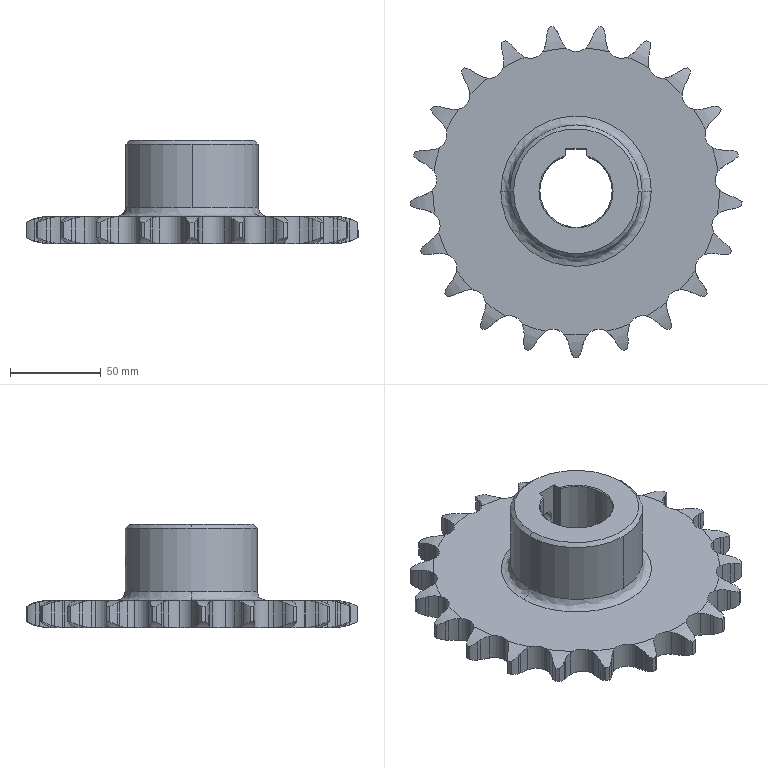Part | SolidWorks | features BaseBody 1 | 1 solid | 246 faces | box 183.758 x 182.894 x 56.916 mm | volume 418597 mm3 | cylinder 144 | plane 50 | spline 46 | cone 6 | commonest cylinder face diameters 26.204 x45 41.431 x44 16.031 x27 183.758 x21 0.5 x2 8.376 x2